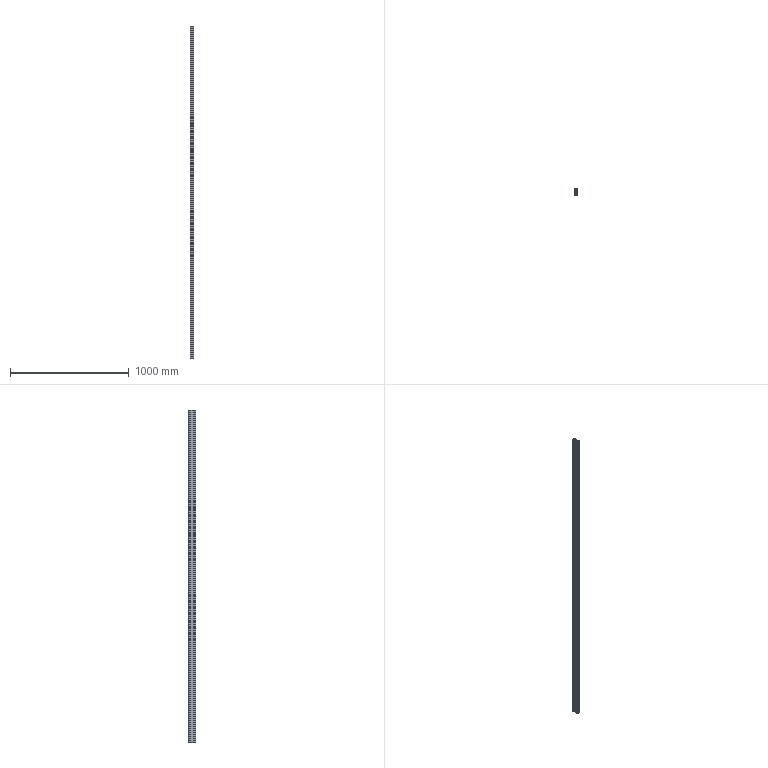Part | SolidWorks | features BaseBody 1 | 1 solid | 169 faces | box 30 x 60 x 2800 mm | volume 1556432 mm3 | plane 118 | cylinder 51 | commonest cylinder face diameters 6.8 x23 1.5 x12 4.2 x8 2 x4 4 x4